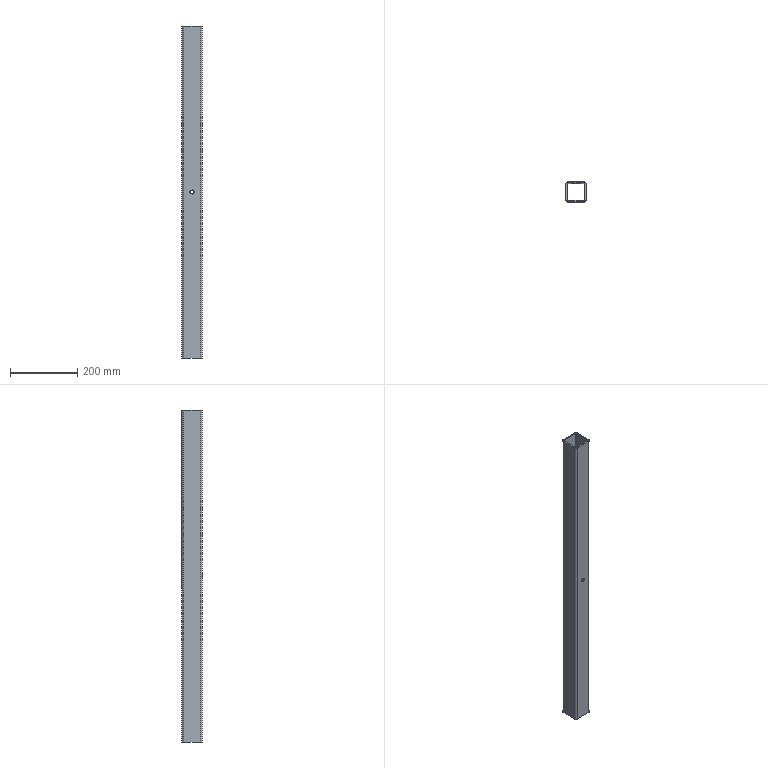Part | STEP file | 750038132 | 1 solid | 30 faces | box 60 x 60 x 985 mm | volume 854437 mm3 | cylinder 16 | plane 10 | cone 4 | commonest cylinder face diameters 12 x8 4 x4 5 x4
STEP:
#1=CARTESIAN_POINT('',(0.,26.,498.5));
#2=VERTEX_POINT('',#1);
#3=CARTESIAN_POINT('',(0.,26.,486.5));
#4=VERTEX_POINT('',#3);
#5=CARTESIAN_POINT('',(0.,26.,492.5));
#6=DIRECTION('',(0.,-1.,0.));
#7=DIRECTION('',(0.,0.,1.));
#8=AXIS2_PLACEMENT_3D('',#5,#6,#7);
#9=CIRCLE('',#8,6.);
#10=EDGE_CURVE('',#2,#4,#9,.T.);
#11=ORIENTED_EDGE('',*,*,#10,.T.);
#12=CARTESIAN_POINT('',(0.,30.,486.5));
#13=VERTEX_POINT('',#12);
#14=CARTESIAN_POINT('',(0.,-36.,486.5));
#15=DIRECTION('',(0.,1.,0.));
#16=VECTOR('',#15,1000.);
#17=LINE('',#14,#16);
#18=EDGE_CURVE('',#4,#13,#17,.T.);
#19=ORIENTED_EDGE('',*,*,#18,.T.);
#20=CARTESIAN_POINT('',(0.,30.,498.5));
#21=VERTEX_POINT('',#20);
#22=CARTESIAN_POINT('',(0.,30.,492.5));
#23=DIRECTION('',(0.,-1.,0.));
#24=DIRECTION('',(0.,0.,1.));
#25=AXIS2_PLACEMENT_3D('',#22,#23,#24);
#26=CIRCLE('',#25,6.);
#27=EDGE_CURVE('',#21,#13,#26,.T.);
#28=ORIENTED_EDGE('',*,*,#27,.F.);
#29=CARTESIAN_POINT('',(0.,-36.,498.5));
#30=DIRECTION('',(0.,1.,0.));
#31=VECTOR('',#30,1000.);
#32=LINE('',#29,#31);
#33=EDGE_CURVE('',#2,#21,#32,.T.);
#34=ORIENTED_EDGE('',*,*,#33,.F.);
#35=EDGE_LOOP('',(#11,#19,#28,#34));
#36=FACE_OUTER_BOUND('',#35,.T.);
#37=CARTESIAN_POINT('',(0.,-36.,492.5));
#38=DIRECTION('',(0.,1.,0.));
#39=DIRECTION('',(0.,0.,1.));
#40=AXIS2_PLACEMENT_3D('',#37,#38,#39);
#41=CYLINDRICAL_SURFACE('',#40,6.);
#42=ADVANCED_FACE('',(#36),#41,.F.);
#43=CARTESIAN_POINT('',(7.5,29.5,457.5));
#44=VERTEX_POINT('',#43);
#45=CARTESIAN_POINT('',(12.5,29.5,457.5));
#46=VERTEX_POINT('',#45);
#47=CARTESIAN_POINT('',(10.,29.5,457.5));
#48=DIRECTION('',(0.,-1.,0.));
#49=DIRECTION('',(1.,0.,0.));
#50=AXIS2_PLACEMENT_3D('',#47,#48,#49);
#51=CIRCLE('',#50,2.5);
#52=EDGE_CURVE('',#44,#46,#51,.T.);
#53=ORIENTED_EDGE('',*,*,#52,.F.);
#54=CARTESIAN_POINT('',(7.5,26.,457.5));
#55=VERTEX_POINT('',#54);
#56=CARTESIAN_POINT('',(7.5,30.,457.5));
#57=DIRECTION('',(0.,-1.,0.));
#58=VECTOR('',#57,1000.);
#59=LINE('',#56,#58);
#60=EDGE_CURVE('',#44,#55,#59,.T.);
#61=ORIENTED_EDGE('',*,*,#60,.T.);
#62=CARTESIAN_POINT('',(12.5,26.,457.5));
#63=VERTEX_POINT('',#62);
#64=CARTESIAN_POINT('',(10.,26.,457.5));
#65=DIRECTION('',(0.,-1.,0.));
#66=DIRECTION('',(1.,0.,0.));
#67=AXIS2_PLACEMENT_3D('',#64,#65,#66);
#68=CIRCLE('',#67,2.5);
#69=EDGE_CURVE('',#55,#63,#68,.T.);
#70=ORIENTED_EDGE('',*,*,#69,.T.);
#71=CARTESIAN_POINT('',(12.5,30.,457.5));
#72=DIRECTION('',(0.,-1.,0.));
#73=VECTOR('',#72,1000.);
#74=LINE('',#71,#73);
#75=EDGE_CURVE('',#46,#63,#74,.T.);
#76=ORIENTED_EDGE('',*,*,#75,.F.);
#77=EDGE_LOOP('',(#53,#61,#70,#76));
#78=FACE_OUTER_BOUND('',#77,.T.);
#79=CARTESIAN_POINT('',(10.,30.,457.5));
#80=DIRECTION('',(0.,-1.,0.));
#81=DIRECTION('',(1.,0.,0.));
#82=AXIS2_PLACEMENT_3D('',#79,#80,#81);
#83=CYLINDRICAL_SURFACE('',#82,2.5);
#84=ADVANCED_FACE('',(#78),#83,.F.);
#85=CARTESIAN_POINT('',(-12.5,29.5,457.5));
#86=VERTEX_POINT('',#85);
#87=CARTESIAN_POINT('',(-7.5,29.5,457.5));
#88=VERTEX_POINT('',#87);
#89=CARTESIAN_POINT('',(-10.,29.5,457.5));
#90=DIRECTION('',(0.,-1.,0.));
#91=DIRECTION('',(1.,0.,0.));
#92=AXIS2_PLACEMENT_3D('',#89,#90,#91);
#93=CIRCLE('',#92,2.5);
#94=EDGE_CURVE('',#86,#88,#93,.T.);
#95=ORIENTED_EDGE('',*,*,#94,.F.);
#96=CARTESIAN_POINT('',(-12.5,26.,457.5));
#97=VERTEX_POINT('',#96);
#98=CARTESIAN_POINT('',(-12.5,30.,457.5));
#99=DIRECTION('',(0.,-1.,0.));
#100=VECTOR('',#99,1000.);
#101=LINE('',#98,#100);
#102=EDGE_CURVE('',#86,#97,#101,.T.);
#103=ORIENTED_EDGE('',*,*,#102,.T.);
#104=CARTESIAN_POINT('',(-7.5,26.,457.5));
#105=VERTEX_POINT('',#104);
#106=CARTESIAN_POINT('',(-10.,26.,457.5));
#107=DIRECTION('',(0.,-1.,0.));
#108=DIRECTION('',(1.,0.,0.));
#109=AXIS2_PLACEMENT_3D('',#106,#107,#108);
#110=CIRCLE('',#109,2.5);
#111=EDGE_CURVE('',#97,#105,#110,.T.);
#112=ORIENTED_EDGE('',*,*,#111,.T.);
#113=CARTESIAN_POINT('',(-7.5,30.,457.5));
#114=DIRECTION('',(0.,-1.,0.));
#115=VECTOR('',#114,1000.);
#116=LINE('',#113,#115);
#117=EDGE_CURVE('',#88,#105,#116,.T.);
#118=ORIENTED_EDGE('',*,*,#117,.F.);
#119=EDGE_LOOP('',(#95,#103,#112,#118));
#120=FACE_OUTER_BOUND('',#119,.T.);
#121=CARTESIAN_POINT('',(-10.,30.,457.5));
#122=DIRECTION('',(0.,-1.,0.));
#123=DIRECTION('',(1.,0.,0.));
#124=AXIS2_PLACEMENT_3D('',#121,#122,#123);
#125=CYLINDRICAL_SURFACE('',#124,2.5);
#126=ADVANCED_FACE('',(#120),#125,.F.);
#127=CARTESIAN_POINT('',(0.,-30.,486.5));
#128=VERTEX_POINT('',#127);
#129=CARTESIAN_POINT('',(0.,-30.,498.5));
#130=VERTEX_POINT('',#129);
#131=CARTESIAN_POINT('',(0.,-30.,492.5));
#132=DIRECTION('',(0.,1.,0.));
#133=DIRECTION('',(0.,0.,1.));
#134=AXIS2_PLACEMENT_3D('',#131,#132,#133);
#135=CIRCLE('',#134,6.);
#136=EDGE_CURVE('',#128,#130,#135,.T.);
#137=ORIENTED_EDGE('',*,*,#136,.F.);
#138=CARTESIAN_POINT('',(0.,-26.,486.5));
#139=VERTEX_POINT('',#138);
#140=CARTESIAN_POINT('',(0.,-36.,486.5));
#141=DIRECTION('',(0.,1.,0.));
#142=VECTOR('',#141,1000.);
#143=LINE('',#140,#142);
#144=EDGE_CURVE('',#128,#139,#143,.T.);
#145=ORIENTED_EDGE('',*,*,#144,.T.);
#146=CARTESIAN_POINT('',(0.,-26.,498.5));
#147=VERTEX_POINT('',#146);
#148=CARTESIAN_POINT('',(0.,-26.,492.5));
#149=DIRECTION('',(0.,1.,0.));
#150=DIRECTION('',(0.,0.,1.));
#151=AXIS2_PLACEMENT_3D('',#148,#149,#150);
#152=CIRCLE('',#151,6.);
#153=EDGE_CURVE('',#139,#147,#152,.T.);
#154=ORIENTED_EDGE('',*,*,#153,.T.);
#155=CARTESIAN_POINT('',(0.,-36.,498.5));
#156=DIRECTION('',(0.,1.,0.));
#157=VECTOR('',#156,1000.);
#158=LINE('',#155,#157);
#159=EDGE_CURVE('',#130,#147,#158,.T.);
#160=ORIENTED_EDGE('',*,*,#159,.F.);
#161=EDGE_LOOP('',(#137,#145,#154,#160));
#162=FACE_OUTER_BOUND('',#161,.T.);
#163=CARTESIAN_POINT('',(0.,-36.,492.5));
#164=DIRECTION('',(0.,1.,0.));
#165=DIRECTION('',(0.,0.,1.));
#166=AXIS2_PLACEMENT_3D('',#163,#164,#165);
#167=CYLINDRICAL_SURFACE('',#166,6.);
#168=ADVANCED_FACE('',(#162),#167,.F.);
#169=ORIENTED_EDGE('',*,*,#52,.T.);
#170=CARTESIAN_POINT('',(13.,30.,457.5));
#171=VERTEX_POINT('',#170);
#172=CARTESIAN_POINT('',(13.,30.,457.5));
#173=DIRECTION('',(0.7071,0.7071,0.));
#174=VECTOR('',#173,1000.);
#175=LINE('',#172,#174);
#176=EDGE_CURVE('',#46,#171,#175,.T.);
#177=ORIENTED_EDGE('',*,*,#176,.T.);
#178=CARTESIAN_POINT('',(7.,30.,457.5));
#179=VERTEX_POINT('',#178);
#180=CARTESIAN_POINT('',(10.,30.,457.5));
#181=DIRECTION('',(0.,-1.,0.));
#182=DIRECTION('',(-1.,0.,0.));
#183=AXIS2_PLACEMENT_3D('',#180,#181,#182);
#184=CIRCLE('',#183,3.);
#185=EDGE_CURVE('',#179,#171,#184,.T.);
#186=ORIENTED_EDGE('',*,*,#185,.F.);
#187=CARTESIAN_POINT('',(7.,30.,457.5));
#188=DIRECTION('',(-0.7071,0.7071,0.));
#189=VECTOR('',#188,1000.);
#190=LINE('',#187,#189);
#191=EDGE_CURVE('',#44,#179,#190,.T.);
#192=ORIENTED_EDGE('',*,*,#191,.F.);
#193=EDGE_LOOP('',(#169,#177,#186,#192));
#194=FACE_OUTER_BOUND('',#193,.T.);
#195=CARTESIAN_POINT('',(10.,30.,457.5));
#196=DIRECTION('',(0.,1.,0.));
#197=DIRECTION('',(-1.,0.,0.));
#198=AXIS2_PLACEMENT_3D('',#195,#196,#197);
#199=CONICAL_SURFACE('',#198,3.,0.7854);
#200=ADVANCED_FACE('',(#194),#199,.F.);
#201=ORIENTED_EDGE('',*,*,#94,.T.);
#202=CARTESIAN_POINT('',(-7.,30.,457.5));
#203=VERTEX_POINT('',#202);
#204=CARTESIAN_POINT('',(-7.,30.,457.5));
#205=DIRECTION('',(0.7071,0.7071,0.));
#206=VECTOR('',#205,1000.);
#207=LINE('',#204,#206);
#208=EDGE_CURVE('',#88,#203,#207,.T.);
#209=ORIENTED_EDGE('',*,*,#208,.T.);
#210=CARTESIAN_POINT('',(-13.,30.,457.5));
#211=VERTEX_POINT('',#210);
#212=CARTESIAN_POINT('',(-10.,30.,457.5));
#213=DIRECTION('',(0.,-1.,0.));
#214=DIRECTION('',(-1.,0.,0.));
#215=AXIS2_PLACEMENT_3D('',#212,#213,#214);
#216=CIRCLE('',#215,3.);
#217=EDGE_CURVE('',#211,#203,#216,.T.);
#218=ORIENTED_EDGE('',*,*,#217,.F.);
#219=CARTESIAN_POINT('',(-13.,30.,457.5));
#220=DIRECTION('',(-0.7071,0.7071,0.));
#221=VECTOR('',#220,1000.);
#222=LINE('',#219,#221);
#223=EDGE_CURVE('',#86,#211,#222,.T.);
#224=ORIENTED_EDGE('',*,*,#223,.F.);
#225=EDGE_LOOP('',(#201,#209,#218,#224));
#226=FACE_OUTER_BOUND('',#225,.T.);
#227=CARTESIAN_POINT('',(-10.,30.,457.5));
#228=DIRECTION('',(0.,1.,0.));
#229=DIRECTION('',(-1.,0.,0.));
#230=AXIS2_PLACEMENT_3D('',#227,#228,#229);
#231=CONICAL_SURFACE('',#230,3.,0.7854);
#232=ADVANCED_FACE('',(#226),#231,.F.);
#233=CARTESIAN_POINT('',(-26.,24.,985.));
#234=VERTEX_POINT('',#233);
#235=CARTESIAN_POINT('',(-26.,24.,0.));
#236=VERTEX_POINT('',#235);
#237=CARTESIAN_POINT('',(-26.,24.,985.));
#238=DIRECTION('',(0.,0.,-1.));
#239=VECTOR('',#238,1000.);
#240=LINE('',#237,#239);
#241=EDGE_CURVE('',#234,#236,#240,.T.);
#242=ORIENTED_EDGE('',*,*,#241,.F.);
#243=CARTESIAN_POINT('',(-26.,-24.,985.));
#244=VERTEX_POINT('',#243);
#245=CARTESIAN_POINT('',(-26.,-24.,985.));
#246=DIRECTION('',(0.,1.,0.));
#247=VECTOR('',#246,1000.);
#248=LINE('',#245,#247);
#249=EDGE_CURVE('',#244,#234,#248,.T.);
#250=ORIENTED_EDGE('',*,*,#249,.F.);
#251=CARTESIAN_POINT('',(-26.,-24.,0.));
#252=VERTEX_POINT('',#251);
#253=CARTESIAN_POINT('',(-26.,-24.,985.));
#254=DIRECTION('',(0.,0.,1.));
#255=VECTOR('',#254,1000.);
#256=LINE('',#253,#255);
#257=EDGE_CURVE('',#252,#244,#256,.T.);
#258=ORIENTED_EDGE('',*,*,#257,.F.);
#259=CARTESIAN_POINT('',(-26.,-24.,0.));
#260=DIRECTION('',(0.,-1.,0.));
#261=VECTOR('',#260,1000.);
#262=LINE('',#259,#261);
#263=EDGE_CURVE('',#236,#252,#262,.T.);
#264=ORIENTED_EDGE('',*,*,#263,.F.);
#265=EDGE_LOOP('',(#242,#250,#258,#264));
#266=FACE_OUTER_BOUND('',#265,.T.);
#267=CARTESIAN_POINT('',(-26.,-24.,985.));
#268=DIRECTION('',(-1.,0.,0.));
#269=DIRECTION('',(0.,-1.,0.));
#270=AXIS2_PLACEMENT_3D('',#267,#268,#269);
#271=PLANE('',#270);
#272=ADVANCED_FACE('',(#266),#271,.F.);
#273=CARTESIAN_POINT('',(26.,24.,0.));
#274=VERTEX_POINT('',#273);
#275=CARTESIAN_POINT('',(24.,26.,0.));
#276=VERTEX_POINT('',#275);
#277=CARTESIAN_POINT('',(24.,24.,0.));
#278=DIRECTION('',(0.,0.,1.));
#279=DIRECTION('',(-1.,0.,0.));
#280=AXIS2_PLACEMENT_3D('',#277,#278,#279);
#281=CIRCLE('',#280,2.);
#282=EDGE_CURVE('',#274,#276,#281,.T.);
#283=ORIENTED_EDGE('',*,*,#282,.T.);
#284=CARTESIAN_POINT('',(-24.,26.,0.));
#285=VERTEX_POINT('',#284);
#286=CARTESIAN_POINT('',(24.,26.,0.));
#287=DIRECTION('',(-1.,0.,0.));
#288=VECTOR('',#287,1000.);
#289=LINE('',#286,#288);
#290=EDGE_CURVE('',#276,#285,#289,.T.);
#291=ORIENTED_EDGE('',*,*,#290,.T.);
#292=CARTESIAN_POINT('',(-24.,24.,0.));
#293=DIRECTION('',(0.,0.,1.));
#294=DIRECTION('',(-1.,0.,0.));
#295=AXIS2_PLACEMENT_3D('',#292,#293,#294);
#296=CIRCLE('',#295,2.);
#297=EDGE_CURVE('',#285,#236,#296,.T.);
#298=ORIENTED_EDGE('',*,*,#297,.T.);
#299=ORIENTED_EDGE('',*,*,#263,.T.);
#300=CARTESIAN_POINT('',(-24.,-26.,0.));
#301=VERTEX_POINT('',#300);
#302=CARTESIAN_POINT('',(-24.,-24.,0.));
#303=DIRECTION('',(0.,0.,1.));
#304=DIRECTION('',(-1.,0.,0.));
#305=AXIS2_PLACEMENT_3D('',#302,#303,#304);
#306=CIRCLE('',#305,2.);
#307=EDGE_CURVE('',#252,#301,#306,.T.);
#308=ORIENTED_EDGE('',*,*,#307,.T.);
#309=CARTESIAN_POINT('',(24.,-26.,0.));
#310=VERTEX_POINT('',#309);
#311=CARTESIAN_POINT('',(24.,-26.,0.));
#312=DIRECTION('',(1.,0.,0.));
#313=VECTOR('',#312,1000.);
#314=LINE('',#311,#313);
#315=EDGE_CURVE('',#301,#310,#314,.T.);
#316=ORIENTED_EDGE('',*,*,#315,.T.);
#317=CARTESIAN_POINT('',(26.,-24.,0.));
#318=VERTEX_POINT('',#317);
#319=CARTESIAN_POINT('',(24.,-24.,0.));
#320=DIRECTION('',(0.,0.,1.));
#321=DIRECTION('',(-1.,0.,0.));
#322=AXIS2_PLACEMENT_3D('',#319,#320,#321);
#323=CIRCLE('',#322,2.);
#324=EDGE_CURVE('',#310,#318,#323,.T.);
#325=ORIENTED_EDGE('',*,*,#324,.T.);
#326=CARTESIAN_POINT('',(26.,-24.,0.));
#327=DIRECTION('',(0.,1.,0.));
#328=VECTOR('',#327,1000.);
#329=LINE('',#326,#328);
#330=EDGE_CURVE('',#318,#274,#329,.T.);
#331=ORIENTED_EDGE('',*,*,#330,.T.);
#332=EDGE_LOOP('',(#283,#291,#298,#299,#308,#316,#325,#331));
#333=FACE_BOUND('',#332,.T.);
#334=CARTESIAN_POINT('',(-24.,30.,0.));
#335=VERTEX_POINT('',#334);
#336=CARTESIAN_POINT('',(24.,30.,0.));
#337=VERTEX_POINT('',#336);
#338=CARTESIAN_POINT('',(24.,30.,0.));
#339=DIRECTION('',(1.,0.,0.));
#340=VECTOR('',#339,1000.);
#341=LINE('',#338,#340);
#342=EDGE_CURVE('',#335,#337,#341,.T.);
#343=ORIENTED_EDGE('',*,*,#342,.T.);
#344=CARTESIAN_POINT('',(30.,24.,0.));
#345=VERTEX_POINT('',#344);
#346=CARTESIAN_POINT('',(24.,24.,0.));
#347=DIRECTION('',(0.,0.,-1.));
#348=DIRECTION('',(-1.,0.,0.));
#349=AXIS2_PLACEMENT_3D('',#346,#347,#348);
#350=CIRCLE('',#349,6.);
#351=EDGE_CURVE('',#337,#345,#350,.T.);
#352=ORIENTED_EDGE('',*,*,#351,.T.);
#353=CARTESIAN_POINT('',(30.,-24.,0.));
#354=VERTEX_POINT('',#353);
#355=CARTESIAN_POINT('',(30.,-24.,0.));
#356=DIRECTION('',(0.,-1.,0.));
#357=VECTOR('',#356,1000.);
#358=LINE('',#355,#357);
#359=EDGE_CURVE('',#345,#354,#358,.T.);
#360=ORIENTED_EDGE('',*,*,#359,.T.);
#361=CARTESIAN_POINT('',(24.,-30.,0.));
#362=VERTEX_POINT('',#361);
#363=CARTESIAN_POINT('',(24.,-24.,0.));
#364=DIRECTION('',(0.,0.,-1.));
#365=DIRECTION('',(-1.,0.,0.));
#366=AXIS2_PLACEMENT_3D('',#363,#364,#365);
#367=CIRCLE('',#366,6.);
#368=EDGE_CURVE('',#354,#362,#367,.T.);
#369=ORIENTED_EDGE('',*,*,#368,.T.);
#370=CARTESIAN_POINT('',(-24.,-30.,0.));
#371=VERTEX_POINT('',#370);
#372=CARTESIAN_POINT('',(24.,-30.,0.));
#373=DIRECTION('',(-1.,0.,0.));
#374=VECTOR('',#373,1000.);
#375=LINE('',#372,#374);
#376=EDGE_CURVE('',#362,#371,#375,.T.);
#377=ORIENTED_EDGE('',*,*,#376,.T.);
#378=CARTESIAN_POINT('',(-30.,-24.,0.));
#379=VERTEX_POINT('',#378);
#380=CARTESIAN_POINT('',(-24.,-24.,0.));
#381=DIRECTION('',(0.,0.,-1.));
#382=DIRECTION('',(-1.,0.,0.));
#383=AXIS2_PLACEMENT_3D('',#380,#381,#382);
#384=CIRCLE('',#383,6.);
#385=EDGE_CURVE('',#371,#379,#384,.T.);
#386=ORIENTED_EDGE('',*,*,#385,.T.);
#387=CARTESIAN_POINT('',(-30.,24.,0.));
#388=VERTEX_POINT('',#387);
#389=CARTESIAN_POINT('',(-30.,-24.,0.));
#390=DIRECTION('',(0.,1.,0.));
#391=VECTOR('',#390,1000.);
#392=LINE('',#389,#391);
#393=EDGE_CURVE('',#379,#388,#392,.T.);
#394=ORIENTED_EDGE('',*,*,#393,.T.);
#395=CARTESIAN_POINT('',(-24.,24.,0.));
#396=DIRECTION('',(0.,0.,-1.));
#397=DIRECTION('',(-1.,0.,0.));
#398=AXIS2_PLACEMENT_3D('',#395,#396,#397);
#399=CIRCLE('',#398,6.);
#400=EDGE_CURVE('',#388,#335,#399,.T.);
#401=ORIENTED_EDGE('',*,*,#400,.T.);
#402=EDGE_LOOP('',(#343,#352,#360,#369,#377,#386,#394,#401));
#403=FACE_OUTER_BOUND('',#402,.T.);
#404=CARTESIAN_POINT('',(24.,-24.,0.));
#405=DIRECTION('',(0.,0.,-1.));
#406=DIRECTION('',(-1.,0.,0.));
#407=AXIS2_PLACEMENT_3D('',#404,#405,#406);
#408=PLANE('',#407);
#409=ADVANCED_FACE('',(#333,#403),#408,.T.);
#410=CARTESIAN_POINT('',(-24.,26.,985.));
#411=VERTEX_POINT('',#410);
#412=CARTESIAN_POINT('',(-24.,26.,985.));
#413=DIRECTION('',(0.,0.,-1.));
#414=VECTOR('',#413,1000.);
#415=LINE('',#412,#414);
#416=EDGE_CURVE('',#411,#285,#415,.T.);
#417=ORIENTED_EDGE('',*,*,#416,.F.);
#418=CARTESIAN_POINT('',(-24.,24.,985.));
#419=DIRECTION('',(0.,0.,-1.));
#420=DIRECTION('',(-1.,0.,0.));
#421=AXIS2_PLACEMENT_3D('',#418,#419,#420);
#422=CIRCLE('',#421,2.);
#423=EDGE_CURVE('',#234,#411,#422,.T.);
#424=ORIENTED_EDGE('',*,*,#423,.F.);
#425=ORIENTED_EDGE('',*,*,#241,.T.);
#426=ORIENTED_EDGE('',*,*,#297,.F.);
#427=EDGE_LOOP('',(#417,#424,#425,#426));
#428=FACE_OUTER_BOUND('',#427,.T.);
#429=CARTESIAN_POINT('',(-24.,24.,985.));
#430=DIRECTION('',(0.,0.,-1.));
#431=DIRECTION('',(-1.,0.,0.));
#432=AXIS2_PLACEMENT_3D('',#429,#430,#431);
#433=CYLINDRICAL_SURFACE('',#432,2.);
#434=ADVANCED_FACE('',(#428),#433,.F.);
#435=CARTESIAN_POINT('',(24.,26.,985.));
#436=VERTEX_POINT('',#435);
#437=CARTESIAN_POINT('',(24.,26.,985.));
#438=DIRECTION('',(-1.,0.,0.));
#439=VECTOR('',#438,1000.);
#440=LINE('',#437,#439);
#441=EDGE_CURVE('',#436,#411,#440,.T.);
#442=ORIENTED_EDGE('',*,*,#441,.F.);
#443=CARTESIAN_POINT('',(26.,24.,985.));
#444=VERTEX_POINT('',#443);
#445=CARTESIAN_POINT('',(24.,24.,985.));
#446=DIRECTION('',(0.,0.,1.));
#447=DIRECTION('',(-1.,0.,0.));
#448=AXIS2_PLACEMENT_3D('',#445,#446,#447);
#449=CIRCLE('',#448,2.);
#450=EDGE_CURVE('',#444,#436,#449,.T.);
#451=ORIENTED_EDGE('',*,*,#450,.F.);
#452=CARTESIAN_POINT('',(26.,-24.,985.));
#453=VERTEX_POINT('',#452);
#454=CARTESIAN_POINT('',(26.,-24.,985.));
#455=DIRECTION('',(0.,1.,0.));
#456=VECTOR('',#455,1000.);
#457=LINE('',#454,#456);
#458=EDGE_CURVE('',#453,#444,#457,.T.);
#459=ORIENTED_EDGE('',*,*,#458,.F.);
#460=CARTESIAN_POINT('',(24.,-26.,985.));
#461=VERTEX_POINT('',#460);
#462=CARTESIAN_POINT('',(24.,-24.,985.));
#463=DIRECTION('',(0.,0.,1.));
#464=DIRECTION('',(-1.,0.,0.));
#465=AXIS2_PLACEMENT_3D('',#462,#463,#464);
#466=CIRCLE('',#465,2.);
#467=EDGE_CURVE('',#461,#453,#466,.T.);
#468=ORIENTED_EDGE('',*,*,#467,.F.);
#469=CARTESIAN_POINT('',(-24.,-26.,985.));
#470=VERTEX_POINT('',#469);
#471=CARTESIAN_POINT('',(24.,-26.,985.));
#472=DIRECTION('',(1.,0.,0.));
#473=VECTOR('',#472,1000.);
#474=LINE('',#471,#473);
#475=EDGE_CURVE('',#470,#461,#474,.T.);
#476=ORIENTED_EDGE('',*,*,#475,.F.);
#477=CARTESIAN_POINT('',(-24.,-24.,985.));
#478=DIRECTION('',(0.,0.,1.));
#479=DIRECTION('',(-1.,0.,0.));
#480=AXIS2_PLACEMENT_3D('',#477,#478,#479);
#481=CIRCLE('',#480,2.);
#482=EDGE_CURVE('',#244,#470,#481,.T.);
#483=ORIENTED_EDGE('',*,*,#482,.F.);
#484=ORIENTED_EDGE('',*,*,#249,.T.);
#485=ORIENTED_EDGE('',*,*,#423,.T.);
#486=EDGE_LOOP('',(#442,#451,#459,#468,#476,#483,#484,#485));
#487=FACE_BOUND('',#486,.T.);
#488=CARTESIAN_POINT('',(24.,30.,985.));
#489=VERTEX_POINT('',#488);
#490=CARTESIAN_POINT('',(30.,24.,985.));
#491=VERTEX_POINT('',#490);
#492=CARTESIAN_POINT('',(24.,24.,985.));
#493=DIRECTION('',(0.,0.,-1.));
#494=DIRECTION('',(-1.,0.,0.));
#495=AXIS2_PLACEMENT_3D('',#492,#493,#494);
#496=CIRCLE('',#495,6.);
#497=EDGE_CURVE('',#489,#491,#496,.T.);
#498=ORIENTED_EDGE('',*,*,#497,.F.);
#499=CARTESIAN_POINT('',(-24.,30.,985.));
#500=VERTEX_POINT('',#499);
#501=CARTESIAN_POINT('',(24.,30.,985.));
#502=DIRECTION('',(1.,0.,0.));
#503=VECTOR('',#502,1000.);
#504=LINE('',#501,#503);
#505=EDGE_CURVE('',#500,#489,#504,.T.);
#506=ORIENTED_EDGE('',*,*,#505,.F.);
#507=CARTESIAN_POINT('',(-30.,24.,985.));
#508=VERTEX_POINT('',#507);
#509=CARTESIAN_POINT('',(-24.,24.,985.));
#510=DIRECTION('',(0.,0.,-1.));
#511=DIRECTION('',(-1.,0.,0.));
#512=AXIS2_PLACEMENT_3D('',#509,#510,#511);
#513=CIRCLE('',#512,6.);
#514=EDGE_CURVE('',#508,#500,#513,.T.);
#515=ORIENTED_EDGE('',*,*,#514,.F.);
#516=CARTESIAN_POINT('',(-30.,-24.,985.));
#517=VERTEX_POINT('',#516);
#518=CARTESIAN_POINT('',(-30.,-24.,985.));
#519=DIRECTION('',(0.,1.,0.));
#520=VECTOR('',#519,1000.);
#521=LINE('',#518,#520);
#522=EDGE_CURVE('',#517,#508,#521,.T.);
#523=ORIENTED_EDGE('',*,*,#522,.F.);
#524=CARTESIAN_POINT('',(-24.,-30.,985.));
#525=VERTEX_POINT('',#524);
#526=CARTESIAN_POINT('',(-24.,-24.,985.));
#527=DIRECTION('',(0.,0.,-1.));
#528=DIRECTION('',(-1.,0.,0.));
#529=AXIS2_PLACEMENT_3D('',#526,#527,#528);
#530=CIRCLE('',#529,6.);
#531=EDGE_CURVE('',#525,#517,#530,.T.);
#532=ORIENTED_EDGE('',*,*,#531,.F.);
#533=CARTESIAN_POINT('',(24.,-30.,985.));
#534=VERTEX_POINT('',#533);
#535=CARTESIAN_POINT('',(24.,-30.,985.));
#536=DIRECTION('',(-1.,0.,0.));
#537=VECTOR('',#536,1000.);
#538=LINE('',#535,#537);
#539=EDGE_CURVE('',#534,#525,#538,.T.);
#540=ORIENTED_EDGE('',*,*,#539,.F.);
#541=CARTESIAN_POINT('',(30.,-24.,985.));
#542=VERTEX_POINT('',#541);
#543=CARTESIAN_POINT('',(24.,-24.,985.));
#544=DIRECTION('',(0.,0.,-1.));
#545=DIRECTION('',(-1.,0.,0.));
#546=AXIS2_PLACEMENT_3D('',#543,#544,#545);
#547=CIRCLE('',#546,6.);
#548=EDGE_CURVE('',#542,#534,#547,.T.);
#549=ORIENTED_EDGE('',*,*,#548,.F.);
#550=CARTESIAN_POINT('',(30.,-24.,985.));
#551=DIRECTION('',(0.,-1.,0.));
#552=VECTOR('',#551,1000.);
#553=LINE('',#550,#552);
#554=EDGE_CURVE('',#491,#542,#553,.T.);
#555=ORIENTED_EDGE('',*,*,#554,.F.);
#556=EDGE_LOOP('',(#498,#506,#515,#523,#532,#540,#549,#555));
#557=FACE_OUTER_BOUND('',#556,.T.);
#558=CARTESIAN_POINT('',(24.,-24.,985.));
#559=DIRECTION('',(0.,0.,-1.));
#560=DIRECTION('',(-1.,0.,0.));
#561=AXIS2_PLACEMENT_3D('',#558,#559,#560);
#562=PLANE('',#561);
#563=ADVANCED_FACE('',(#487,#557),#562,.F.);
#564=ORIENTED_EDGE('',*,*,#257,.T.);
#565=ORIENTED_EDGE('',*,*,#482,.T.);
#566=CARTESIAN_POINT('',(-24.,-26.,985.));
#567=DIRECTION('',(0.,0.,1.));
#568=VECTOR('',#567,1000.);
#569=LINE('',#566,#568);
#570=EDGE_CURVE('',#301,#470,#569,.T.);
#571=ORIENTED_EDGE('',*,*,#570,.F.);
#572=ORIENTED_EDGE('',*,*,#307,.F.);
#573=EDGE_LOOP('',(#564,#565,#571,#572));
#574=FACE_OUTER_BOUND('',#573,.T.);
#575=CARTESIAN_POINT('',(-24.,-24.,985.));
#576=DIRECTION('',(0.,0.,-1.));
#577=DIRECTION('',(-1.,0.,0.));
#578=AXIS2_PLACEMENT_3D('',#575,#576,#577);
#579=CYLINDRICAL_SURFACE('',#578,2.);
#580=ADVANCED_FACE('',(#574),#579,.F.);
#581=CARTESIAN_POINT('',(24.,26.,985.));
#582=DIRECTION('',(0.,0.,-1.));
#583=VECTOR('',#582,1000.);
#584=LINE('',#581,#583);
#585=EDGE_CURVE('',#436,#276,#584,.T.);
#586=ORIENTED_EDGE('',*,*,#585,.F.);
#587=ORIENTED_EDGE('',*,*,#441,.T.);
#588=ORIENTED_EDGE('',*,*,#416,.T.);
#589=ORIENTED_EDGE('',*,*,#290,.F.);
#590=EDGE_LOOP('',(#586,#587,#588,#589));
#591=FACE_OUTER_BOUND('',#590,.T.);
#592=ORIENTED_EDGE('',*,*,#10,.F.);
#593=CARTESIAN_POINT('',(0.,26.,492.5));
#594=DIRECTION('',(0.,-1.,0.));
#595=DIRECTION('',(0.,0.,1.));
#596=AXIS2_PLACEMENT_3D('',#593,#594,#595);
#597=CIRCLE('',#596,6.);
#598=EDGE_CURVE('',#4,#2,#597,.T.);
#599=ORIENTED_EDGE('',*,*,#598,.F.);
#600=EDGE_LOOP('',(#592,#599));
#601=FACE_BOUND('',#600,.T.);
#602=CARTESIAN_POINT('',(10.,26.,457.5));
#603=DIRECTION('',(0.,-1.,0.));
#604=DIRECTION('',(1.,0.,0.));
#605=AXIS2_PLACEMENT_3D('',#602,#603,#604);
#606=CIRCLE('',#605,2.5);
#607=EDGE_CURVE('',#63,#55,#606,.T.);
#608=ORIENTED_EDGE('',*,*,#607,.F.);
#609=ORIENTED_EDGE('',*,*,#69,.F.);
#610=EDGE_LOOP('',(#608,#609));
#611=FACE_BOUND('',#610,.T.);
#612=CARTESIAN_POINT('',(-10.,26.,457.5));
#613=DIRECTION('',(0.,-1.,0.));
#614=DIRECTION('',(1.,0.,0.));
#615=AXIS2_PLACEMENT_3D('',#612,#613,#614);
#616=CIRCLE('',#615,2.5);
#617=EDGE_CURVE('',#105,#97,#616,.T.);
#618=ORIENTED_EDGE('',*,*,#617,.F.);
#619=ORIENTED_EDGE('',*,*,#111,.F.);
#620=EDGE_LOOP('',(#618,#619));
#621=FACE_BOUND('',#620,.T.);
#622=CARTESIAN_POINT('',(-24.,26.,985.));
#623=DIRECTION('',(0.,1.,0.));
#624=DIRECTION('',(0.,0.,1.));
#625=AXIS2_PLACEMENT_3D('',#622,#623,#624);
#626=PLANE('',#625);
#627=ADVANCED_FACE('',(#591,#601,#611,#621),#626,.F.);
#628=CARTESIAN_POINT('',(26.,24.,985.));
#629=DIRECTION('',(0.,0.,-1.));
#630=VECTOR('',#629,1000.);
#631=LINE('',#628,#630);
#632=EDGE_CURVE('',#444,#274,#631,.T.);
#633=ORIENTED_EDGE('',*,*,#632,.F.);
#634=ORIENTED_EDGE('',*,*,#450,.T.);
#635=ORIENTED_EDGE('',*,*,#585,.T.);
#636=ORIENTED_EDGE('',*,*,#282,.F.);
#637=EDGE_LOOP('',(#633,#634,#635,#636));
#638=FACE_OUTER_BOUND('',#637,.T.);
#639=CARTESIAN_POINT('',(24.,24.,985.));
#640=DIRECTION('',(0.,0.,-1.));
#641=DIRECTION('',(-1.,0.,0.));
#642=AXIS2_PLACEMENT_3D('',#639,#640,#641);
#643=CYLINDRICAL_SURFACE('',#642,2.);
#644=ADVANCED_FACE('',(#638),#643,.F.);
#645=CARTESIAN_POINT('',(26.,-24.,985.));
#646=DIRECTION('',(0.,0.,-1.));
#647=VECTOR('',#646,1000.);
#648=LINE('',#645,#647);
#649=EDGE_CURVE('',#453,#318,#648,.T.);
#650=ORIENTED_EDGE('',*,*,#649,.F.);
#651=ORIENTED_EDGE('',*,*,#458,.T.);
#652=ORIENTED_EDGE('',*,*,#632,.T.);
#653=ORIENTED_EDGE('',*,*,#330,.F.);
#654=EDGE_LOOP('',(#650,#651,#652,#653));
#655=FACE_OUTER_BOUND('',#654,.T.);
#656=CARTESIAN_POINT('',(26.,24.,985.));
#657=DIRECTION('',(1.,0.,0.));
#658=DIRECTION('',(0.,0.,-1.));
#659=AXIS2_PLACEMENT_3D('',#656,#657,#658);
#660=PLANE('',#659);
#661=ADVANCED_FACE('',(#655),#660,.F.);
#662=CARTESIAN_POINT('',(24.,-26.,985.));
#663=DIRECTION('',(0.,0.,-1.));
#664=VECTOR('',#663,1000.);
#665=LINE('',#662,#664);
#666=EDGE_CURVE('',#461,#310,#665,.T.);
#667=ORIENTED_EDGE('',*,*,#666,.F.);
#668=ORIENTED_EDGE('',*,*,#467,.T.);
#669=ORIENTED_EDGE('',*,*,#649,.T.);
#670=ORIENTED_EDGE('',*,*,#324,.F.);
#671=EDGE_LOOP('',(#667,#668,#669,#670));
#672=FACE_OUTER_BOUND('',#671,.T.);
#673=CARTESIAN_POINT('',(24.,-24.,985.));
#674=DIRECTION('',(0.,0.,-1.));
#675=DIRECTION('',(-1.,0.,0.));
#676=AXIS2_PLACEMENT_3D('',#673,#674,#675);
#677=CYLINDRICAL_SURFACE('',#676,2.);
#678=ADVANCED_FACE('',(#672),#677,.F.);
#679=ORIENTED_EDGE('',*,*,#570,.T.);
#680=ORIENTED_EDGE('',*,*,#475,.T.);
#681=ORIENTED_EDGE('',*,*,#666,.T.);
#682=ORIENTED_EDGE('',*,*,#315,.F.);
#683=EDGE_LOOP('',(#679,#680,#681,#682));
#684=FACE_OUTER_BOUND('',#683,.T.);
#685=CARTESIAN_POINT('',(0.,-26.,492.5));
#686=DIRECTION('',(0.,1.,0.));
#687=DIRECTION('',(0.,0.,1.));
#688=AXIS2_PLACEMENT_3D('',#685,#686,#687);
#689=CIRCLE('',#688,6.);
#690=EDGE_CURVE('',#147,#139,#689,.T.);
#691=ORIENTED_EDGE('',*,*,#690,.F.);
#692=ORIENTED_EDGE('',*,*,#153,.F.);
#693=EDGE_LOOP('',(#691,#692));
#694=FACE_BOUND('',#693,.T.);
#695=CARTESIAN_POINT('',(24.,-26.,985.));
#696=DIRECTION('',(0.,-1.,0.));
#697=DIRECTION('',(0.,0.,-1.));
#698=AXIS2_PLACEMENT_3D('',#695,#696,#697);
#699=PLANE('',#698);
#700=ADVANCED_FACE('',(#684,#694),#699,.F.);
#701=ORIENTED_EDGE('',*,*,#497,.T.);
#702=CARTESIAN_POINT('',(30.,24.,985.));
#703=DIRECTION('',(0.,0.,-1.));
#704=VECTOR('',#703,1000.);
#705=LINE('',#702,#704);
#706=EDGE_CURVE('',#491,#345,#705,.T.);
#707=ORIENTED_EDGE('',*,*,#706,.T.);
#708=ORIENTED_EDGE('',*,*,#351,.F.);
#709=CARTESIAN_POINT('',(24.,30.,985.));
#710=DIRECTION('',(0.,0.,1.));
#711=VECTOR('',#710,1000.);
#712=LINE('',#709,#711);
#713=EDGE_CURVE('',#337,#489,#712,.T.);
#714=ORIENTED_EDGE('',*,*,#713,.T.);
#715=EDGE_LOOP('',(#701,#707,#708,#714));
#716=FACE_OUTER_BOUND('',#715,.T.);
#717=CARTESIAN_POINT('',(24.,24.,985.));
#718=DIRECTION('',(0.,0.,-1.));
#719=DIRECTION('',(-1.,0.,0.));
#720=AXIS2_PLACEMENT_3D('',#717,#718,#719);
#721=CYLINDRICAL_SURFACE('',#720,6.);
#722=ADVANCED_FACE('',(#716),#721,.T.);
#723=ORIENTED_EDGE('',*,*,#505,.T.);
#724=ORIENTED_EDGE('',*,*,#713,.F.);
#725=ORIENTED_EDGE('',*,*,#342,.F.);
#726=CARTESIAN_POINT('',(-24.,30.,985.));
#727=DIRECTION('',(0.,0.,1.));
#728=VECTOR('',#727,1000.);
#729=LINE('',#726,#728);
#730=EDGE_CURVE('',#335,#500,#729,.T.);
#731=ORIENTED_EDGE('',*,*,#730,.T.);
#732=EDGE_LOOP('',(#723,#724,#725,#731));
#733=FACE_OUTER_BOUND('',#732,.T.);
#734=ORIENTED_EDGE('',*,*,#27,.T.);
#735=CARTESIAN_POINT('',(0.,30.,492.5));
#736=DIRECTION('',(0.,-1.,0.));
#737=DIRECTION('',(0.,0.,1.));
#738=AXIS2_PLACEMENT_3D('',#735,#736,#737);
#739=CIRCLE('',#738,6.);
#740=EDGE_CURVE('',#13,#21,#739,.T.);
#741=ORIENTED_EDGE('',*,*,#740,.T.);
#742=EDGE_LOOP('',(#734,#741));
#743=FACE_BOUND('',#742,.T.);
#744=ORIENTED_EDGE('',*,*,#185,.T.);
#745=CARTESIAN_POINT('',(10.,30.,457.5));
#746=DIRECTION('',(0.,-1.,0.));
#747=DIRECTION('',(-1.,0.,0.));
#748=AXIS2_PLACEMENT_3D('',#745,#746,#747);
#749=CIRCLE('',#748,3.);
#750=EDGE_CURVE('',#171,#179,#749,.T.);
#751=ORIENTED_EDGE('',*,*,#750,.T.);
#752=EDGE_LOOP('',(#744,#751));
#753=FACE_BOUND('',#752,.T.);
#754=ORIENTED_EDGE('',*,*,#217,.T.);
#755=CARTESIAN_POINT('',(-10.,30.,457.5));
#756=DIRECTION('',(0.,-1.,0.));
#757=DIRECTION('',(-1.,0.,0.));
#758=AXIS2_PLACEMENT_3D('',#755,#756,#757);
#759=CIRCLE('',#758,3.);
#760=EDGE_CURVE('',#203,#211,#759,.T.);
#761=ORIENTED_EDGE('',*,*,#760,.T.);
#762=EDGE_LOOP('',(#754,#761));
#763=FACE_BOUND('',#762,.T.);
#764=CARTESIAN_POINT('',(-24.,30.,985.));
#765=DIRECTION('',(0.,1.,0.));
#766=DIRECTION('',(-1.,0.,0.));
#767=AXIS2_PLACEMENT_3D('',#764,#765,#766);
#768=PLANE('',#767);
#769=ADVANCED_FACE('',(#733,#743,#753,#763),#768,.T.);
#770=ORIENTED_EDGE('',*,*,#514,.T.);
#771=ORIENTED_EDGE('',*,*,#730,.F.);
#772=ORIENTED_EDGE('',*,*,#400,.F.);
#773=CARTESIAN_POINT('',(-30.,24.,985.));
#774=DIRECTION('',(0.,0.,1.));
#775=VECTOR('',#774,1000.);
#776=LINE('',#773,#775);
#777=EDGE_CURVE('',#388,#508,#776,.T.);
#778=ORIENTED_EDGE('',*,*,#777,.T.);
#779=EDGE_LOOP('',(#770,#771,#772,#778));
#780=FACE_OUTER_BOUND('',#779,.T.);
#781=CARTESIAN_POINT('',(-24.,24.,985.));
#782=DIRECTION('',(0.,0.,-1.));
#783=DIRECTION('',(-1.,0.,0.));
#784=AXIS2_PLACEMENT_3D('',#781,#782,#783);
#785=CYLINDRICAL_SURFACE('',#784,6.);
#786=ADVANCED_FACE('',(#780),#785,.T.);
#787=ORIENTED_EDGE('',*,*,#522,.T.);
#788=ORIENTED_EDGE('',*,*,#777,.F.);
#789=ORIENTED_EDGE('',*,*,#393,.F.);
#790=CARTESIAN_POINT('',(-30.,-24.,985.));
#791=DIRECTION('',(0.,0.,1.));
#792=VECTOR('',#791,1000.);
#793=LINE('',#790,#792);
#794=EDGE_CURVE('',#379,#517,#793,.T.);
#795=ORIENTED_EDGE('',*,*,#794,.T.);
#796=EDGE_LOOP('',(#787,#788,#789,#795));
#797=FACE_OUTER_BOUND('',#796,.T.);
#798=CARTESIAN_POINT('',(-30.,-24.,985.));
#799=DIRECTION('',(-1.,0.,0.));
#800=DIRECTION('',(0.,-1.,0.));
#801=AXIS2_PLACEMENT_3D('',#798,#799,#800);
#802=PLANE('',#801);
#803=ADVANCED_FACE('',(#797),#802,.T.);
#804=ORIENTED_EDGE('',*,*,#531,.T.);
#805=ORIENTED_EDGE('',*,*,#794,.F.);
#806=ORIENTED_EDGE('',*,*,#385,.F.);
#807=CARTESIAN_POINT('',(-24.,-30.,985.));
#808=DIRECTION('',(0.,0.,1.));
#809=VECTOR('',#808,1000.);
#810=LINE('',#807,#809);
#811=EDGE_CURVE('',#371,#525,#810,.T.);
#812=ORIENTED_EDGE('',*,*,#811,.T.);
#813=EDGE_LOOP('',(#804,#805,#806,#812));
#814=FACE_OUTER_BOUND('',#813,.T.);
#815=CARTESIAN_POINT('',(-24.,-24.,985.));
#816=DIRECTION('',(0.,0.,-1.));
#817=DIRECTION('',(-1.,0.,0.));
#818=AXIS2_PLACEMENT_3D('',#815,#816,#817);
#819=CYLINDRICAL_SURFACE('',#818,6.);
#820=ADVANCED_FACE('',(#814),#819,.T.);
#821=ORIENTED_EDGE('',*,*,#539,.T.);
#822=ORIENTED_EDGE('',*,*,#811,.F.);
#823=ORIENTED_EDGE('',*,*,#376,.F.);
#824=CARTESIAN_POINT('',(24.,-30.,985.));
#825=DIRECTION('',(0.,0.,1.));
#826=VECTOR('',#825,1000.);
#827=LINE('',#824,#826);
#828=EDGE_CURVE('',#362,#534,#827,.T.);
#829=ORIENTED_EDGE('',*,*,#828,.T.);
#830=EDGE_LOOP('',(#821,#822,#823,#829));
#831=FACE_OUTER_BOUND('',#830,.T.);
#832=CARTESIAN_POINT('',(0.,-30.,492.5));
#833=DIRECTION('',(0.,1.,0.));
#834=DIRECTION('',(0.,0.,1.));
#835=AXIS2_PLACEMENT_3D('',#832,#833,#834);
#836=CIRCLE('',#835,6.);
#837=EDGE_CURVE('',#130,#128,#836,.T.);
#838=ORIENTED_EDGE('',*,*,#837,.T.);
#839=ORIENTED_EDGE('',*,*,#136,.T.);
#840=EDGE_LOOP('',(#838,#839));
#841=FACE_BOUND('',#840,.T.);
#842=CARTESIAN_POINT('',(24.,-30.,985.));
#843=DIRECTION('',(0.,-1.,0.));
#844=DIRECTION('',(1.,0.,0.));
#845=AXIS2_PLACEMENT_3D('',#842,#843,#844);
#846=PLANE('',#845);
#847=ADVANCED_FACE('',(#831,#841),#846,.T.);
#848=ORIENTED_EDGE('',*,*,#548,.T.);
#849=ORIENTED_EDGE('',*,*,#828,.F.);
#850=ORIENTED_EDGE('',*,*,#368,.F.);
#851=CARTESIAN_POINT('',(30.,-24.,985.));
#852=DIRECTION('',(0.,0.,1.));
#853=VECTOR('',#852,1000.);
#854=LINE('',#851,#853);
#855=EDGE_CURVE('',#354,#542,#854,.T.);
#856=ORIENTED_EDGE('',*,*,#855,.T.);
#857=EDGE_LOOP('',(#848,#849,#850,#856));
#858=FACE_OUTER_BOUND('',#857,.T.);
#859=CARTESIAN_POINT('',(24.,-24.,985.));
#860=DIRECTION('',(0.,0.,-1.));
#861=DIRECTION('',(-1.,0.,0.));
#862=AXIS2_PLACEMENT_3D('',#859,#860,#861);
#863=CYLINDRICAL_SURFACE('',#862,6.);
#864=ADVANCED_FACE('',(#858),#863,.T.);
#865=ORIENTED_EDGE('',*,*,#554,.T.);
#866=ORIENTED_EDGE('',*,*,#855,.F.);
#867=ORIENTED_EDGE('',*,*,#359,.F.);
#868=ORIENTED_EDGE('',*,*,#706,.F.);
#869=EDGE_LOOP('',(#865,#866,#867,#868));
#870=FACE_OUTER_BOUND('',#869,.T.);
#871=CARTESIAN_POINT('',(30.,24.,985.));
#872=DIRECTION('',(1.,0.,0.));
#873=DIRECTION('',(0.,0.,-1.));
#874=AXIS2_PLACEMENT_3D('',#871,#872,#873);
#875=PLANE('',#874);
#876=ADVANCED_FACE('',(#870),#875,.T.);
#877=ORIENTED_EDGE('',*,*,#18,.F.);
#878=ORIENTED_EDGE('',*,*,#598,.T.);
#879=ORIENTED_EDGE('',*,*,#33,.T.);
#880=ORIENTED_EDGE('',*,*,#740,.F.);
#881=EDGE_LOOP('',(#877,#878,#879,#880));
#882=FACE_OUTER_BOUND('',#881,.T.);
#883=CARTESIAN_POINT('',(0.,-36.,492.5));
#884=DIRECTION('',(0.,1.,0.));
#885=DIRECTION('',(0.,0.,1.));
#886=AXIS2_PLACEMENT_3D('',#883,#884,#885);
#887=CYLINDRICAL_SURFACE('',#886,6.);
#888=ADVANCED_FACE('',(#882),#887,.F.);
#889=ORIENTED_EDGE('',*,*,#60,.F.);
#890=CARTESIAN_POINT('',(10.,29.5,457.5));
#891=DIRECTION('',(0.,-1.,0.));
#892=DIRECTION('',(1.,0.,0.));
#893=AXIS2_PLACEMENT_3D('',#890,#891,#892);
#894=CIRCLE('',#893,2.5);
#895=EDGE_CURVE('',#46,#44,#894,.T.);
#896=ORIENTED_EDGE('',*,*,#895,.F.);
#897=ORIENTED_EDGE('',*,*,#75,.T.);
#898=ORIENTED_EDGE('',*,*,#607,.T.);
#899=EDGE_LOOP('',(#889,#896,#897,#898));
#900=FACE_OUTER_BOUND('',#899,.T.);
#901=CARTESIAN_POINT('',(10.,30.,457.5));
#902=DIRECTION('',(0.,-1.,0.));
#903=DIRECTION('',(1.,0.,0.));
#904=AXIS2_PLACEMENT_3D('',#901,#902,#903);
#905=CYLINDRICAL_SURFACE('',#904,2.5);
#906=ADVANCED_FACE('',(#900),#905,.F.);
#907=ORIENTED_EDGE('',*,*,#102,.F.);
#908=CARTESIAN_POINT('',(-10.,29.5,457.5));
#909=DIRECTION('',(0.,-1.,0.));
#910=DIRECTION('',(1.,0.,0.));
#911=AXIS2_PLACEMENT_3D('',#908,#909,#910);
#912=CIRCLE('',#911,2.5);
#913=EDGE_CURVE('',#88,#86,#912,.T.);
#914=ORIENTED_EDGE('',*,*,#913,.F.);
#915=ORIENTED_EDGE('',*,*,#117,.T.);
#916=ORIENTED_EDGE('',*,*,#617,.T.);
#917=EDGE_LOOP('',(#907,#914,#915,#916));
#918=FACE_OUTER_BOUND('',#917,.T.);
#919=CARTESIAN_POINT('',(-10.,30.,457.5));
#920=DIRECTION('',(0.,-1.,0.));
#921=DIRECTION('',(1.,0.,0.));
#922=AXIS2_PLACEMENT_3D('',#919,#920,#921);
#923=CYLINDRICAL_SURFACE('',#922,2.5);
#924=ADVANCED_FACE('',(#918),#923,.F.);
#925=ORIENTED_EDGE('',*,*,#144,.F.);
#926=ORIENTED_EDGE('',*,*,#837,.F.);
#927=ORIENTED_EDGE('',*,*,#159,.T.);
#928=ORIENTED_EDGE('',*,*,#690,.T.);
#929=EDGE_LOOP('',(#925,#926,#927,#928));
#930=FACE_OUTER_BOUND('',#929,.T.);
#931=CARTESIAN_POINT('',(0.,-36.,492.5));
#932=DIRECTION('',(0.,1.,0.));
#933=DIRECTION('',(0.,0.,1.));
#934=AXIS2_PLACEMENT_3D('',#931,#932,#933);
#935=CYLINDRICAL_SURFACE('',#934,6.);
#936=ADVANCED_FACE('',(#930),#935,.F.);
#937=ORIENTED_EDGE('',*,*,#176,.F.);
#938=ORIENTED_EDGE('',*,*,#895,.T.);
#939=ORIENTED_EDGE('',*,*,#191,.T.);
#940=ORIENTED_EDGE('',*,*,#750,.F.);
#941=EDGE_LOOP('',(#937,#938,#939,#940));
#942=FACE_OUTER_BOUND('',#941,.T.);
#943=CARTESIAN_POINT('',(10.,30.,457.5));
#944=DIRECTION('',(0.,1.,0.));
#945=DIRECTION('',(-1.,0.,0.));
#946=AXIS2_PLACEMENT_3D('',#943,#944,#945);
#947=CONICAL_SURFACE('',#946,3.,0.7854);
#948=ADVANCED_FACE('',(#942),#947,.F.);
#949=ORIENTED_EDGE('',*,*,#208,.F.);
#950=ORIENTED_EDGE('',*,*,#913,.T.);
#951=ORIENTED_EDGE('',*,*,#223,.T.);
#952=ORIENTED_EDGE('',*,*,#760,.F.);
#953=EDGE_LOOP('',(#949,#950,#951,#952));
#954=FACE_OUTER_BOUND('',#953,.T.);
#955=CARTESIAN_POINT('',(-10.,30.,457.5));
#956=DIRECTION('',(0.,1.,0.));
#957=DIRECTION('',(-1.,0.,0.));
#958=AXIS2_PLACEMENT_3D('',#955,#956,#957);
#959=CONICAL_SURFACE('',#958,3.,0.7854);
#960=ADVANCED_FACE('',(#954),#959,.F.);
#961=CLOSED_SHELL('',(#42,#84,#126,#168,#200,#232,#272,#409,#434,#563,#580,#627,#644,#661,#678,#700,#722,#769,#786,#803,#820,#847,#864,#876,#888,#906,#924,#936,#948,#960));
#962=MANIFOLD_SOLID_BREP('',#961);
#963=CARTESIAN_POINT('',(0.,0.,0.));
#964=DIRECTION('',(0.,0.,1.));
#965=DIRECTION('',(1.,0.,0.));
#966=AXIS2_PLACEMENT_3D('',#963,#964,#965);
#967=(LENGTH_UNIT()NAMED_UNIT(*)SI_UNIT(.MILLI.,.METRE.));
#968=UNCERTAINTY_MEASURE_WITH_UNIT(LENGTH_MEASURE(0.00001),#967,'','');
#969=(NAMED_UNIT(*)PLANE_ANGLE_UNIT()SI_UNIT($,.RADIAN.));
#970=(NAMED_UNIT(*)SI_UNIT($,.STERADIAN.)SOLID_ANGLE_UNIT());
#971=(GEOMETRIC_REPRESENTATION_CONTEXT(3)GLOBAL_UNCERTAINTY_ASSIGNED_CONTEXT((#968))GLOBAL_UNIT_ASSIGNED_CONTEXT((#967,#969,#970))REPRESENTATION_CONTEXT('',''));
#972=ADVANCED_BREP_SHAPE_REPRESENTATION('',(#962,#966),#971);